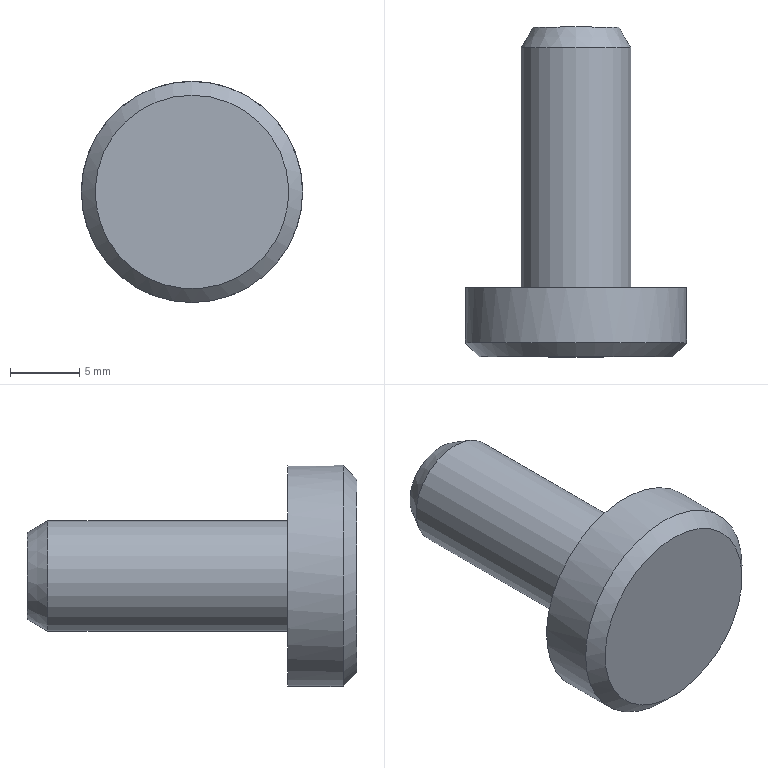Part | STEP file | STOP-PIN_id318_x_t | 1 solid | 7 faces | box 16 x 23.859 x 16 mm | volume 1914 mm3 | plane 3 | cone 2 | cylinder 2 | commonest cylinder face diameters 8 x1 16 x1
STEP:
#1=CARTESIAN_POINT('',(94.,-255.5,-33.));
#2=VERTEX_POINT('',#1);
#3=CARTESIAN_POINT('',(94.,-255.5,-40.));
#4=DIRECTION('',(0.,1.,0.));
#5=DIRECTION('',(0.,0.,1.));
#6=AXIS2_PLACEMENT_3D('',#3,#4,#5);
#7=CIRCLE('',#6,7.);
#8=EDGE_CURVE('',#2,#2,#7,.T.);
#9=ORIENTED_EDGE('',*,*,#8,.F.);
#10=EDGE_LOOP('',(#9));
#11=FACE_OUTER_BOUND('',#10,.T.);
#12=CARTESIAN_POINT('',(94.,-255.5,-40.));
#13=DIRECTION('',(0.,-1.,0.));
#14=DIRECTION('',(0.,0.,-1.));
#15=AXIS2_PLACEMENT_3D('',#12,#13,#14);
#16=PLANE('',#15);
#17=ADVANCED_FACE('',(#11),#16,.T.);
#18=ORIENTED_EDGE('',*,*,#8,.T.);
#19=EDGE_LOOP('',(#18));
#20=FACE_BOUND('',#19,.T.);
#21=CARTESIAN_POINT('',(94.,-254.5,-48.));
#22=VERTEX_POINT('',#21);
#23=CARTESIAN_POINT('',(94.,-254.5,-40.));
#24=DIRECTION('',(0.,1.,0.));
#25=DIRECTION('',(0.,0.,-1.));
#26=AXIS2_PLACEMENT_3D('',#23,#24,#25);
#27=CIRCLE('',#26,8.);
#28=EDGE_CURVE('',#22,#22,#27,.T.);
#29=ORIENTED_EDGE('',*,*,#28,.F.);
#30=EDGE_LOOP('',(#29));
#31=FACE_BOUND('',#30,.T.);
#32=CARTESIAN_POINT('',(94.,-254.5,-40.));
#33=DIRECTION('',(0.,1.,0.));
#34=DIRECTION('',(0.,0.,1.));
#35=AXIS2_PLACEMENT_3D('',#32,#33,#34);
#36=CONICAL_SURFACE('',#35,8.,45.);
#37=ADVANCED_FACE('',(#20,#31),#36,.T.);
#38=CARTESIAN_POINT('',(94.,-231.641,-43.134));
#39=VERTEX_POINT('',#38);
#40=CARTESIAN_POINT('',(94.,-231.641,-40.));
#41=DIRECTION('',(0.,-1.,0.));
#42=DIRECTION('',(0.,0.,-1.));
#43=AXIS2_PLACEMENT_3D('',#40,#41,#42);
#44=CIRCLE('',#43,3.134);
#45=EDGE_CURVE('',#39,#39,#44,.T.);
#46=ORIENTED_EDGE('',*,*,#45,.F.);
#47=EDGE_LOOP('',(#46));
#48=FACE_OUTER_BOUND('',#47,.T.);
#49=CARTESIAN_POINT('',(94.,-231.641,-40.));
#50=DIRECTION('',(0.,-1.,0.));
#51=DIRECTION('',(0.,0.,-1.));
#52=AXIS2_PLACEMENT_3D('',#49,#50,#51);
#53=PLANE('',#52);
#54=ADVANCED_FACE('',(#48),#53,.F.);
#55=ORIENTED_EDGE('',*,*,#28,.T.);
#56=EDGE_LOOP('',(#55));
#57=FACE_BOUND('',#56,.T.);
#58=CARTESIAN_POINT('',(94.,-250.5,-48.));
#59=VERTEX_POINT('',#58);
#60=CARTESIAN_POINT('',(94.,-250.5,-40.));
#61=DIRECTION('',(0.,-1.,0.));
#62=DIRECTION('',(0.,0.,-1.));
#63=AXIS2_PLACEMENT_3D('',#60,#61,#62);
#64=CIRCLE('',#63,8.);
#65=EDGE_CURVE('',#59,#59,#64,.T.);
#66=ORIENTED_EDGE('',*,*,#65,.T.);
#67=EDGE_LOOP('',(#66));
#68=FACE_BOUND('',#67,.T.);
#69=CARTESIAN_POINT('',(94.,-256.693,-40.));
#70=DIRECTION('',(0.,-1.,0.));
#71=DIRECTION('',(0.,0.,-1.));
#72=AXIS2_PLACEMENT_3D('',#69,#70,#71);
#73=CYLINDRICAL_SURFACE('',#72,8.);
#74=ADVANCED_FACE('',(#57,#68),#73,.T.);
#75=CARTESIAN_POINT('',(94.,-233.141,-44.));
#76=VERTEX_POINT('',#75);
#77=CARTESIAN_POINT('',(94.,-233.141,-40.));
#78=DIRECTION('',(0.,-1.,0.));
#79=DIRECTION('',(0.,0.,-1.));
#80=AXIS2_PLACEMENT_3D('',#77,#78,#79);
#81=CIRCLE('',#80,4.);
#82=EDGE_CURVE('',#76,#76,#81,.T.);
#83=ORIENTED_EDGE('',*,*,#82,.F.);
#84=EDGE_LOOP('',(#83));
#85=FACE_BOUND('',#84,.T.);
#86=ORIENTED_EDGE('',*,*,#45,.T.);
#87=EDGE_LOOP('',(#86));
#88=FACE_BOUND('',#87,.T.);
#89=CARTESIAN_POINT('',(94.,-233.141,-40.));
#90=DIRECTION('',(0.,-1.,0.));
#91=DIRECTION('',(0.,0.,-1.));
#92=AXIS2_PLACEMENT_3D('',#89,#90,#91);
#93=CONICAL_SURFACE('',#92,4.,30.);
#94=ADVANCED_FACE('',(#85,#88),#93,.T.);
#95=CARTESIAN_POINT('',(94.,-250.5,-44.));
#96=VERTEX_POINT('',#95);
#97=CARTESIAN_POINT('',(94.,-250.5,-40.));
#98=DIRECTION('',(0.,1.,0.));
#99=DIRECTION('',(0.,0.,-1.));
#100=AXIS2_PLACEMENT_3D('',#97,#98,#99);
#101=CIRCLE('',#100,4.);
#102=EDGE_CURVE('',#96,#96,#101,.T.);
#103=ORIENTED_EDGE('',*,*,#102,.F.);
#104=EDGE_LOOP('',(#103));
#105=FACE_BOUND('',#104,.T.);
#106=ORIENTED_EDGE('',*,*,#65,.F.);
#107=EDGE_LOOP('',(#106));
#108=FACE_BOUND('',#107,.T.);
#109=CARTESIAN_POINT('',(94.,-250.5,-40.));
#110=DIRECTION('',(0.,-1.,0.));
#111=DIRECTION('',(0.,0.,-1.));
#112=AXIS2_PLACEMENT_3D('',#109,#110,#111);
#113=PLANE('',#112);
#114=ADVANCED_FACE('',(#105,#108),#113,.F.);
#115=ORIENTED_EDGE('',*,*,#102,.T.);
#116=EDGE_LOOP('',(#115));
#117=FACE_BOUND('',#116,.T.);
#118=ORIENTED_EDGE('',*,*,#82,.T.);
#119=EDGE_LOOP('',(#118));
#120=FACE_BOUND('',#119,.T.);
#121=CARTESIAN_POINT('',(94.,-256.693,-40.));
#122=DIRECTION('',(0.,-1.,0.));
#123=DIRECTION('',(0.,0.,-1.));
#124=AXIS2_PLACEMENT_3D('',#121,#122,#123);
#125=CYLINDRICAL_SURFACE('',#124,4.);
#126=ADVANCED_FACE('',(#117,#120),#125,.T.);
#127=CLOSED_SHELL('',(#17,#37,#54,#74,#94,#114,#126));
#128=MANIFOLD_SOLID_BREP('',#127);
#129=(LENGTH_UNIT()NAMED_UNIT(*)SI_UNIT(.MILLI.,.METRE.));
#130=UNCERTAINTY_MEASURE_WITH_UNIT(LENGTH_MEASURE(0.00002),#129,'','');
#131=(NAMED_UNIT(*)PLANE_ANGLE_UNIT()SI_UNIT($,.RADIAN.));
#132=PLANE_ANGLE_MEASURE_WITH_UNIT(PLANE_ANGLE_MEASURE(0.01745),#131);
#133=DIMENSIONAL_EXPONENTS(0.,0.,0.,0.,0.,0.,0.);
#134=(CONVERSION_BASED_UNIT('DEGREE',#132)NAMED_UNIT(#133)PLANE_ANGLE_UNIT());
#135=(NAMED_UNIT(*)SI_UNIT($,.STERADIAN.)SOLID_ANGLE_UNIT());
#136=(GEOMETRIC_REPRESENTATION_CONTEXT(3)GLOBAL_UNCERTAINTY_ASSIGNED_CONTEXT((#130))GLOBAL_UNIT_ASSIGNED_CONTEXT((#129,#134,#135))REPRESENTATION_CONTEXT('',''));
#137=ADVANCED_BREP_SHAPE_REPRESENTATION('',(#128),#136);